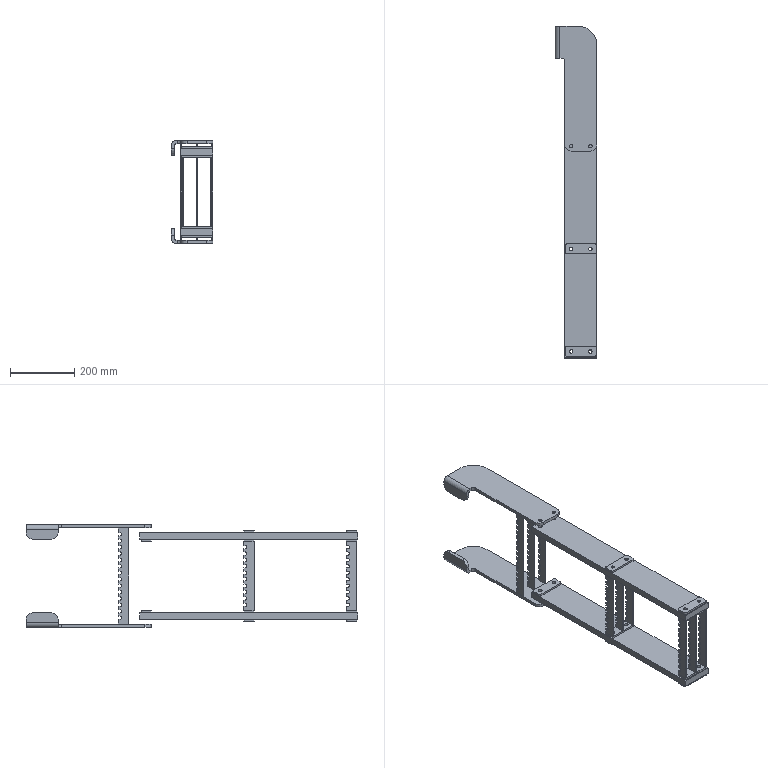Part | SolidWorks | 23 solids | 682 faces | box 130 x 1035 x 320 mm | volume 3924769 mm3 | plane 460 | cylinder 222 | commonest cylinder face diameters 10 x126 11 x72 12 x8 40 x8 8 x2 20 x2